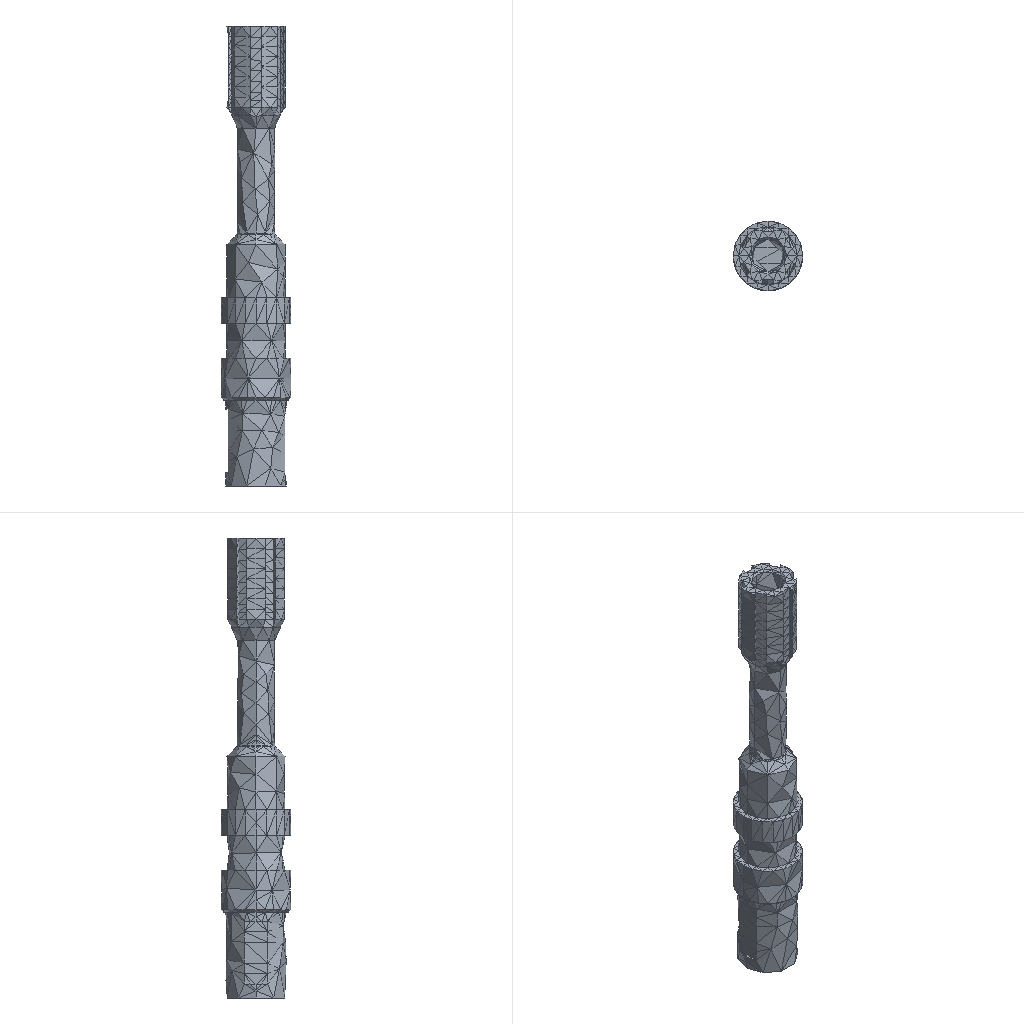Simulation study | ansys workbench
Set-up summary:
category,name,step,type,value,unit,region
solver,ansys_mapdl
solver,version,,,22.1
solver,version,,,22.1
units,MPA,,stated
analysis,deck1,,modal,modal
load_step,requested,,,1
analysis,nlgeom,,,False
mesh,nodes,,,5069
mesh,elements,,,2686
element_type,ANSYS 187 (type 1),,solid,2686
load,load commands in deck,,count,0
bc,support commands in deck,,count,0
analysis,deck2,,static,static
load_step,requested,,,1
analysis,nlgeom,,,False
mesh,nodes,,,5070
mesh,elements,,,2932
element_type,ANSYS 187 (type 1),,solid,2686
element_type,ANSYS 174 (type 2),,contact,246
element_type,ANSYS 170 (type 3),,target,0
load,load commands in deck,,count,3
bc,support commands in deck,,count,1
named_set,_FIXEDSU,,component
material,1,,in results
material,1,,in results
check,setup vs results,,match
check,setup vs results,,match,results also hold 0 node(s) and 1 element(s) the deck makes with ['EN']; those were not compared; 1 node(s) the solver created internally for pilot nodes (solve.out) are in the results only
Results summary:
result,analysis,,,modal
result,last_loadstep,,,1
result,primary field,,,displacement
result,analysis,,,static
result,last_loadstep,,,1
result,primary field,,,displacement
result,reaction total,1,FX,1.1e-05,N
result,reaction total,1,FY,-4e-06,N
result,reaction total,1,FZ,-5e-06,N
result,mass,,,0.000642,"NMM: mm, ton, N, s, mV, mA, degC"